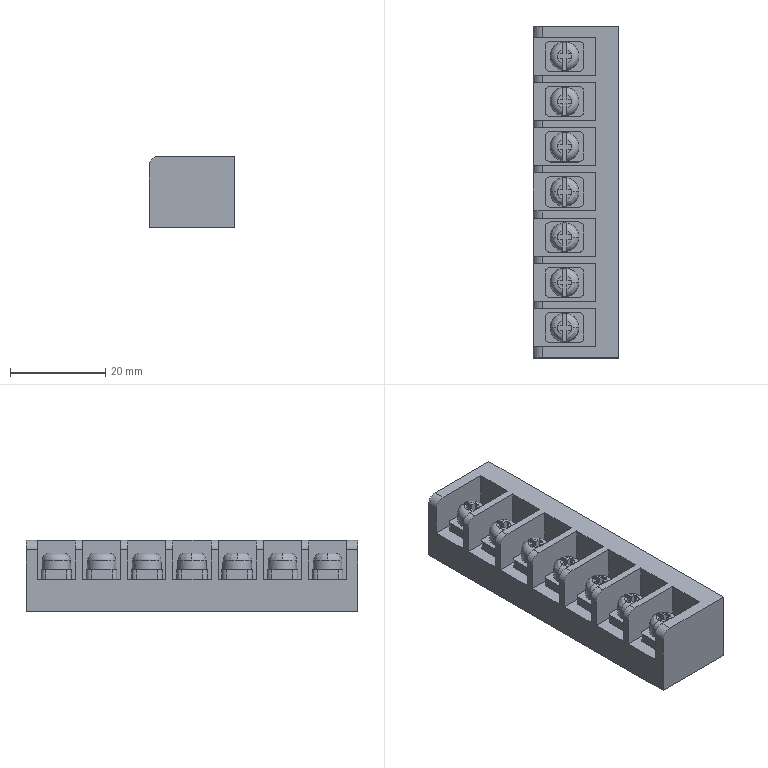Part | STEP file | LRS-150-12_X2_5F00517375-151317 | 1 solid | 260 faces | box 18 x 69.7 x 15 mm | volume 13984 mm3 | plane 188 | cylinder 50 | spline 16 | torus 6 | commonest cylinder face diameters 2 x28 6 x14 4 x8